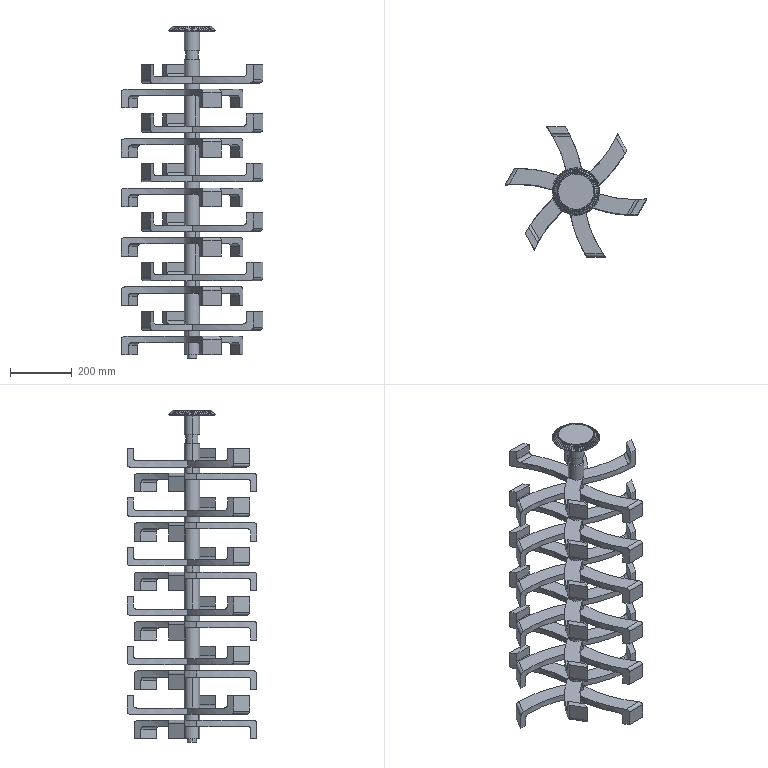Part | SolidWorks | 1 solid | 436 faces | box 458.731 x 420 x 1075 mm | volume 11323145 mm3 | cylinder 176 | plane 138 | cone 62 | spline 60 | commonest cylinder face diameters 20 x72 700 x36 800 x36 50 x28 30 x2 40 x2